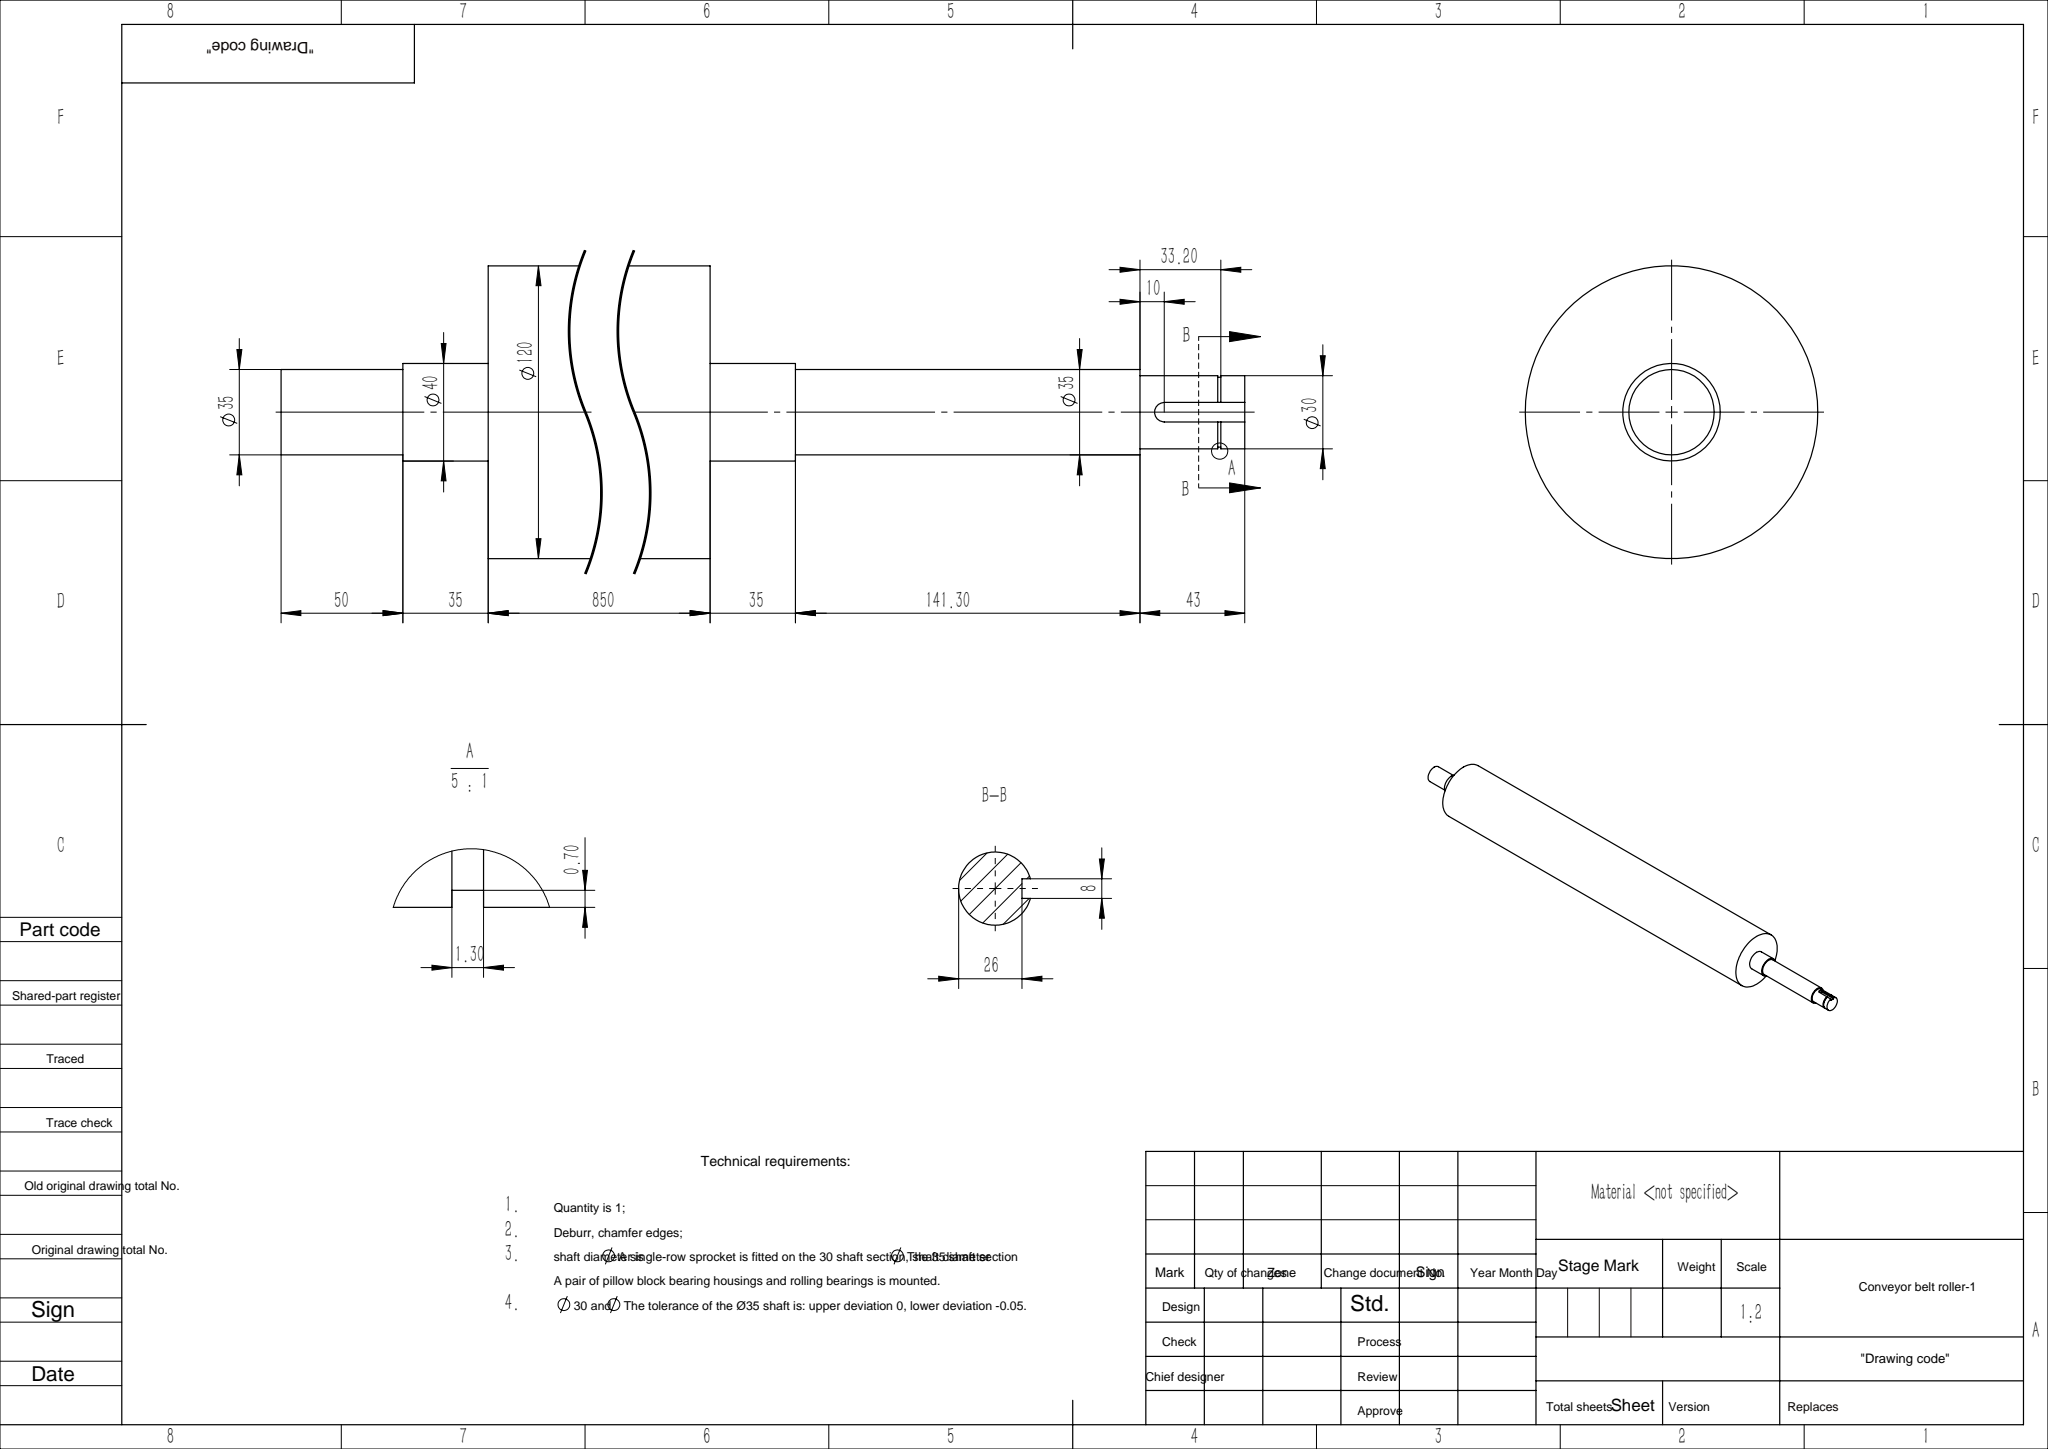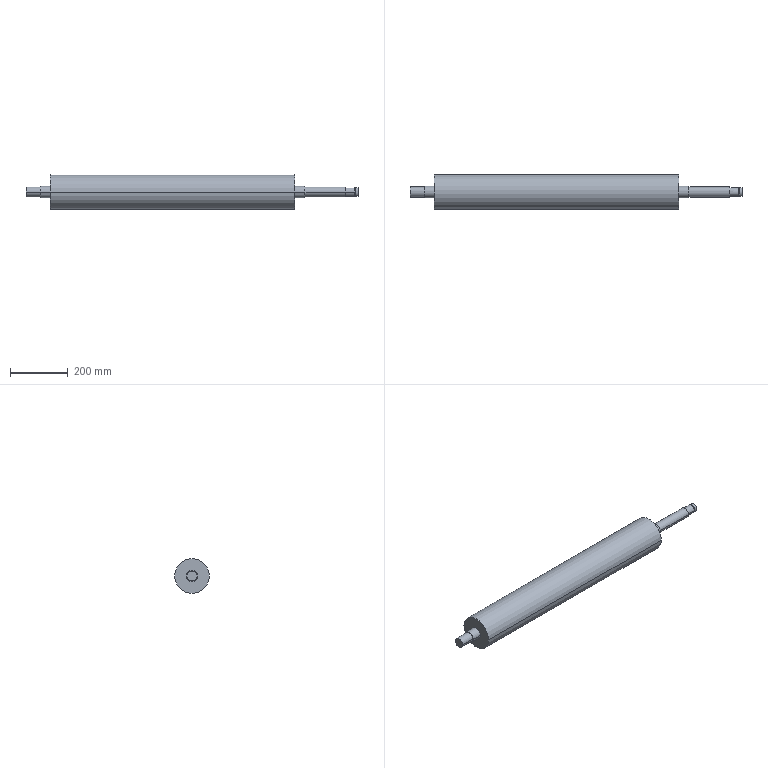Part | SolidWorks | features ICE 2, Revolution 1 | 1 solid | 28 faces | box 1154 x 120 x 120 mm | volume 9914503 mm3 | cylinder 16 | plane 12 | commonest cylinder face diameters 35 x4 40 x4 30 x3 8 x2 120 x2 28.6 x1
STEP:
#1=CARTESIAN_POINT('',(1117.3,11.,0.));
#2=VERTEX_POINT('',#1);
#3=CARTESIAN_POINT('',(1121.3,11.,4.));
#4=VERTEX_POINT('',#3);
#5=CARTESIAN_POINT('',(1121.3,11.,0.));
#6=DIRECTION('',(0.,1.,0.));
#7=DIRECTION('',(-1.,0.,0.));
#8=AXIS2_PLACEMENT_3D('',#5,#6,#7);
#9=CIRCLE('',#8,4.);
#10=EDGE_CURVE('',#2,#4,#9,.T.);
#11=ORIENTED_EDGE('',*,*,#10,.F.);
#12=CARTESIAN_POINT('',(1117.3,15.,0.));
#13=VERTEX_POINT('',#12);
#14=CARTESIAN_POINT('',(1117.3,11.,0.));
#15=DIRECTION('',(0.,1.,0.));
#16=VECTOR('',#15,1000.);
#17=LINE('',#14,#16);
#18=EDGE_CURVE('',#2,#13,#17,.T.);
#19=ORIENTED_EDGE('',*,*,#18,.T.);
#20=CARTESIAN_POINT('',(1121.3,14.457,4.));
#21=VERTEX_POINT('',#20);
#22=CARTESIAN_POINT('',(1117.3,15.,0.));
#23=CARTESIAN_POINT('',(1117.3,15.,0.262));
#24=CARTESIAN_POINT('',(1117.326,14.993,0.5282));
#25=CARTESIAN_POINT('',(1117.429,14.966,1.042));
#26=CARTESIAN_POINT('',(1117.505,14.946,1.292));
#27=CARTESIAN_POINT('',(1117.808,14.871,2.02));
#28=CARTESIAN_POINT('',(1118.102,14.802,2.459));
#29=CARTESIAN_POINT('',(1118.657,14.695,3.014));
#30=CARTESIAN_POINT('',(1118.857,14.66,3.178));
#31=CARTESIAN_POINT('',(1119.289,14.594,3.467));
#32=CARTESIAN_POINT('',(1119.523,14.564,3.593));
#33=CARTESIAN_POINT('',(1120.005,14.513,3.794));
#34=CARTESIAN_POINT('',(1120.254,14.492,3.87));
#35=CARTESIAN_POINT('',(1120.769,14.464,3.973));
#36=CARTESIAN_POINT('',(1121.035,14.457,4.));
#37=CARTESIAN_POINT('',(1121.3,14.457,4.));
#38=B_SPLINE_CURVE_WITH_KNOTS('',3,(#22,#23,#24,#25,#26,#27,#28,#29,#30,#31,#32,#33,#34,#35,#36,#37),.UNSPECIFIED.,.F.,.F.,(4,2,2,2,2,2,2,4),(0.006283,0.007068,0.007852,0.009421,0.01021,0.01099,0.01177,0.01256),.UNSPECIFIED.);
#39=EDGE_CURVE('',#13,#21,#38,.T.);
#40=ORIENTED_EDGE('',*,*,#39,.T.);
#41=CARTESIAN_POINT('',(1121.3,11.,4.));
#42=DIRECTION('',(0.,1.,0.));
#43=VECTOR('',#42,1000.);
#44=LINE('',#41,#43);
#45=EDGE_CURVE('',#4,#21,#44,.T.);
#46=ORIENTED_EDGE('',*,*,#45,.F.);
#47=EDGE_LOOP('',(#11,#19,#40,#46));
#48=FACE_OUTER_BOUND('',#47,.T.);
#49=CARTESIAN_POINT('',(1121.3,11.,0.));
#50=DIRECTION('',(0.,1.,0.));
#51=DIRECTION('',(-1.,0.,0.));
#52=AXIS2_PLACEMENT_3D('',#49,#50,#51);
#53=CYLINDRICAL_SURFACE('',#52,4.);
#54=ADVANCED_FACE('',(#48),#53,.F.);
#55=CARTESIAN_POINT('',(970.,17.5,0.));
#56=VERTEX_POINT('',#55);
#57=CARTESIAN_POINT('',(970.,-17.5,0.));
#58=VERTEX_POINT('',#57);
#59=CARTESIAN_POINT('',(970.,0.,0.));
#60=DIRECTION('',(1.,0.,0.));
#61=DIRECTION('',(0.,1.,0.));
#62=AXIS2_PLACEMENT_3D('',#59,#60,#61);
#63=CIRCLE('',#62,17.5);
#64=EDGE_CURVE('',#56,#58,#63,.T.);
#65=ORIENTED_EDGE('',*,*,#64,.T.);
#66=CARTESIAN_POINT('',(1111.3,-17.5,0.));
#67=VERTEX_POINT('',#66);
#68=CARTESIAN_POINT('',(1154.3,-17.5,0.));
#69=DIRECTION('',(1.,0.,0.));
#70=VECTOR('',#69,1000.);
#71=LINE('',#68,#70);
#72=EDGE_CURVE('',#58,#67,#71,.T.);
#73=ORIENTED_EDGE('',*,*,#72,.T.);
#74=CARTESIAN_POINT('',(1111.3,17.5,0.));
#75=VERTEX_POINT('',#74);
#76=CARTESIAN_POINT('',(1111.3,0.,0.));
#77=DIRECTION('',(1.,0.,0.));
#78=DIRECTION('',(0.,1.,0.));
#79=AXIS2_PLACEMENT_3D('',#76,#77,#78);
#80=CIRCLE('',#79,17.5);
#81=EDGE_CURVE('',#75,#67,#80,.T.);
#82=ORIENTED_EDGE('',*,*,#81,.F.);
#83=CARTESIAN_POINT('',(1154.3,17.5,0.));
#84=DIRECTION('',(1.,0.,0.));
#85=VECTOR('',#84,1000.);
#86=LINE('',#83,#85);
#87=EDGE_CURVE('',#56,#75,#86,.T.);
#88=ORIENTED_EDGE('',*,*,#87,.F.);
#89=EDGE_LOOP('',(#65,#73,#82,#88));
#90=FACE_OUTER_BOUND('',#89,.T.);
#91=CARTESIAN_POINT('',(1154.3,0.,0.));
#92=DIRECTION('',(1.,0.,0.));
#93=DIRECTION('',(0.,1.,0.));
#94=AXIS2_PLACEMENT_3D('',#91,#92,#93);
#95=CYLINDRICAL_SURFACE('',#94,17.5);
#96=ADVANCED_FACE('',(#90),#95,.T.);
#97=CARTESIAN_POINT('',(935.,20.,0.));
#98=VERTEX_POINT('',#97);
#99=CARTESIAN_POINT('',(935.,-20.,0.));
#100=VERTEX_POINT('',#99);
#101=CARTESIAN_POINT('',(935.,0.,0.));
#102=DIRECTION('',(1.,0.,0.));
#103=DIRECTION('',(0.,1.,0.));
#104=AXIS2_PLACEMENT_3D('',#101,#102,#103);
#105=CIRCLE('',#104,20.);
#106=EDGE_CURVE('',#98,#100,#105,.T.);
#107=ORIENTED_EDGE('',*,*,#106,.T.);
#108=CARTESIAN_POINT('',(970.,-20.,0.));
#109=VERTEX_POINT('',#108);
#110=CARTESIAN_POINT('',(1154.3,-20.,0.));
#111=DIRECTION('',(1.,0.,0.));
#112=VECTOR('',#111,1000.);
#113=LINE('',#110,#112);
#114=EDGE_CURVE('',#100,#109,#113,.T.);
#115=ORIENTED_EDGE('',*,*,#114,.T.);
#116=CARTESIAN_POINT('',(970.,20.,0.));
#117=VERTEX_POINT('',#116);
#118=CARTESIAN_POINT('',(970.,0.,0.));
#119=DIRECTION('',(1.,0.,0.));
#120=DIRECTION('',(0.,1.,0.));
#121=AXIS2_PLACEMENT_3D('',#118,#119,#120);
#122=CIRCLE('',#121,20.);
#123=EDGE_CURVE('',#117,#109,#122,.T.);
#124=ORIENTED_EDGE('',*,*,#123,.F.);
#125=CARTESIAN_POINT('',(1154.3,20.,0.));
#126=DIRECTION('',(1.,0.,0.));
#127=VECTOR('',#126,1000.);
#128=LINE('',#125,#127);
#129=EDGE_CURVE('',#98,#117,#128,.T.);
#130=ORIENTED_EDGE('',*,*,#129,.F.);
#131=EDGE_LOOP('',(#107,#115,#124,#130));
#132=FACE_OUTER_BOUND('',#131,.T.);
#133=CARTESIAN_POINT('',(1154.3,0.,0.));
#134=DIRECTION('',(1.,0.,0.));
#135=DIRECTION('',(0.,1.,0.));
#136=AXIS2_PLACEMENT_3D('',#133,#134,#135);
#137=CYLINDRICAL_SURFACE('',#136,20.);
#138=ADVANCED_FACE('',(#132),#137,.T.);
#139=CARTESIAN_POINT('',(85.,60.,0.));
#140=VERTEX_POINT('',#139);
#141=CARTESIAN_POINT('',(85.,-60.,0.));
#142=VERTEX_POINT('',#141);
#143=CARTESIAN_POINT('',(85.,0.,0.));
#144=DIRECTION('',(1.,0.,0.));
#145=DIRECTION('',(0.,1.,0.));
#146=AXIS2_PLACEMENT_3D('',#143,#144,#145);
#147=CIRCLE('',#146,60.);
#148=EDGE_CURVE('',#140,#142,#147,.T.);
#149=ORIENTED_EDGE('',*,*,#148,.T.);
#150=CARTESIAN_POINT('',(935.,-60.,0.));
#151=VERTEX_POINT('',#150);
#152=CARTESIAN_POINT('',(1154.3,-60.,0.));
#153=DIRECTION('',(1.,0.,0.));
#154=VECTOR('',#153,1000.);
#155=LINE('',#152,#154);
#156=EDGE_CURVE('',#142,#151,#155,.T.);
#157=ORIENTED_EDGE('',*,*,#156,.T.);
#158=CARTESIAN_POINT('',(935.,60.,0.));
#159=VERTEX_POINT('',#158);
#160=CARTESIAN_POINT('',(935.,0.,0.));
#161=DIRECTION('',(1.,0.,0.));
#162=DIRECTION('',(0.,1.,0.));
#163=AXIS2_PLACEMENT_3D('',#160,#161,#162);
#164=CIRCLE('',#163,60.);
#165=EDGE_CURVE('',#159,#151,#164,.T.);
#166=ORIENTED_EDGE('',*,*,#165,.F.);
#167=CARTESIAN_POINT('',(1154.3,60.,0.));
#168=DIRECTION('',(1.,0.,0.));
#169=VECTOR('',#168,1000.);
#170=LINE('',#167,#169);
#171=EDGE_CURVE('',#140,#159,#170,.T.);
#172=ORIENTED_EDGE('',*,*,#171,.F.);
#173=EDGE_LOOP('',(#149,#157,#166,#172));
#174=FACE_OUTER_BOUND('',#173,.T.);
#175=CARTESIAN_POINT('',(1154.3,0.,0.));
#176=DIRECTION('',(1.,0.,0.));
#177=DIRECTION('',(0.,1.,0.));
#178=AXIS2_PLACEMENT_3D('',#175,#176,#177);
#179=CYLINDRICAL_SURFACE('',#178,60.);
#180=ADVANCED_FACE('',(#174),#179,.T.);
#181=CARTESIAN_POINT('',(50.,20.,0.));
#182=VERTEX_POINT('',#181);
#183=CARTESIAN_POINT('',(50.,-20.,0.));
#184=VERTEX_POINT('',#183);
#185=CARTESIAN_POINT('',(50.,0.,0.));
#186=DIRECTION('',(1.,0.,0.));
#187=DIRECTION('',(0.,1.,0.));
#188=AXIS2_PLACEMENT_3D('',#185,#186,#187);
#189=CIRCLE('',#188,20.);
#190=EDGE_CURVE('',#182,#184,#189,.T.);
#191=ORIENTED_EDGE('',*,*,#190,.T.);
#192=CARTESIAN_POINT('',(85.,-20.,0.));
#193=VERTEX_POINT('',#192);
#194=CARTESIAN_POINT('',(1154.3,-20.,0.));
#195=DIRECTION('',(1.,0.,0.));
#196=VECTOR('',#195,1000.);
#197=LINE('',#194,#196);
#198=EDGE_CURVE('',#184,#193,#197,.T.);
#199=ORIENTED_EDGE('',*,*,#198,.T.);
#200=CARTESIAN_POINT('',(85.,20.,0.));
#201=VERTEX_POINT('',#200);
#202=CARTESIAN_POINT('',(85.,0.,0.));
#203=DIRECTION('',(1.,0.,0.));
#204=DIRECTION('',(0.,1.,0.));
#205=AXIS2_PLACEMENT_3D('',#202,#203,#204);
#206=CIRCLE('',#205,20.);
#207=EDGE_CURVE('',#201,#193,#206,.T.);
#208=ORIENTED_EDGE('',*,*,#207,.F.);
#209=CARTESIAN_POINT('',(1154.3,20.,0.));
#210=DIRECTION('',(1.,0.,0.));
#211=VECTOR('',#210,1000.);
#212=LINE('',#209,#211);
#213=EDGE_CURVE('',#182,#201,#212,.T.);
#214=ORIENTED_EDGE('',*,*,#213,.F.);
#215=EDGE_LOOP('',(#191,#199,#208,#214));
#216=FACE_OUTER_BOUND('',#215,.T.);
#217=CARTESIAN_POINT('',(1154.3,0.,0.));
#218=DIRECTION('',(1.,0.,0.));
#219=DIRECTION('',(0.,1.,0.));
#220=AXIS2_PLACEMENT_3D('',#217,#218,#219);
#221=CYLINDRICAL_SURFACE('',#220,20.);
#222=ADVANCED_FACE('',(#216),#221,.T.);
#223=CARTESIAN_POINT('',(0.,17.5,0.));
#224=VERTEX_POINT('',#223);
#225=CARTESIAN_POINT('',(0.,-17.5,0.));
#226=VERTEX_POINT('',#225);
#227=CARTESIAN_POINT('',(0.,0.,0.));
#228=DIRECTION('',(1.,0.,0.));
#229=DIRECTION('',(0.,1.,0.));
#230=AXIS2_PLACEMENT_3D('',#227,#228,#229);
#231=CIRCLE('',#230,17.5);
#232=EDGE_CURVE('',#224,#226,#231,.T.);
#233=ORIENTED_EDGE('',*,*,#232,.T.);
#234=CARTESIAN_POINT('',(50.,-17.5,0.));
#235=VERTEX_POINT('',#234);
#236=CARTESIAN_POINT('',(1154.3,-17.5,0.));
#237=DIRECTION('',(1.,0.,0.));
#238=VECTOR('',#237,1000.);
#239=LINE('',#236,#238);
#240=EDGE_CURVE('',#226,#235,#239,.T.);
#241=ORIENTED_EDGE('',*,*,#240,.T.);
#242=CARTESIAN_POINT('',(50.,17.5,0.));
#243=VERTEX_POINT('',#242);
#244=CARTESIAN_POINT('',(50.,0.,0.));
#245=DIRECTION('',(1.,0.,0.));
#246=DIRECTION('',(0.,1.,0.));
#247=AXIS2_PLACEMENT_3D('',#244,#245,#246);
#248=CIRCLE('',#247,17.5);
#249=EDGE_CURVE('',#243,#235,#248,.T.);
#250=ORIENTED_EDGE('',*,*,#249,.F.);
#251=CARTESIAN_POINT('',(1154.3,17.5,0.));
#252=DIRECTION('',(1.,0.,0.));
#253=VECTOR('',#252,1000.);
#254=LINE('',#251,#253);
#255=EDGE_CURVE('',#224,#243,#254,.T.);
#256=ORIENTED_EDGE('',*,*,#255,.F.);
#257=EDGE_LOOP('',(#233,#241,#250,#256));
#258=FACE_OUTER_BOUND('',#257,.T.);
#259=CARTESIAN_POINT('',(1154.3,0.,0.));
#260=DIRECTION('',(1.,0.,0.));
#261=DIRECTION('',(0.,1.,0.));
#262=AXIS2_PLACEMENT_3D('',#259,#260,#261);
#263=CYLINDRICAL_SURFACE('',#262,17.5);
#264=ADVANCED_FACE('',(#258),#263,.T.);
#265=CARTESIAN_POINT('',(1111.3,15.,0.));
#266=VERTEX_POINT('',#265);
#267=CARTESIAN_POINT('',(1111.3,-15.,0.));
#268=VERTEX_POINT('',#267);
#269=CARTESIAN_POINT('',(1111.3,0.,0.));
#270=DIRECTION('',(1.,0.,0.));
#271=DIRECTION('',(0.,1.,0.));
#272=AXIS2_PLACEMENT_3D('',#269,#270,#271);
#273=CIRCLE('',#272,15.);
#274=EDGE_CURVE('',#266,#268,#273,.T.);
#275=ORIENTED_EDGE('',*,*,#274,.T.);
#276=CARTESIAN_POINT('',(1143.2,-15.,0.));
#277=VERTEX_POINT('',#276);
#278=CARTESIAN_POINT('',(1154.3,-15.,0.));
#279=DIRECTION('',(1.,0.,0.));
#280=VECTOR('',#279,1000.);
#281=LINE('',#278,#280);
#282=EDGE_CURVE('',#268,#277,#281,.T.);
#283=ORIENTED_EDGE('',*,*,#282,.T.);
#284=CARTESIAN_POINT('',(1143.2,14.457,4.));
#285=VERTEX_POINT('',#284);
#286=CARTESIAN_POINT('',(1143.2,0.,0.));
#287=DIRECTION('',(1.,0.,0.));
#288=DIRECTION('',(0.,1.,0.));
#289=AXIS2_PLACEMENT_3D('',#286,#287,#288);
#290=CIRCLE('',#289,15.);
#291=EDGE_CURVE('',#285,#277,#290,.T.);
#292=ORIENTED_EDGE('',*,*,#291,.F.);
#293=CARTESIAN_POINT('',(1154.3,14.457,4.));
#294=DIRECTION('',(1.,0.,0.));
#295=VECTOR('',#294,1000.);
#296=LINE('',#293,#295);
#297=EDGE_CURVE('',#21,#285,#296,.T.);
#298=ORIENTED_EDGE('',*,*,#297,.F.);
#299=ORIENTED_EDGE('',*,*,#39,.F.);
#300=CARTESIAN_POINT('',(1154.3,15.,0.));
#301=DIRECTION('',(1.,0.,0.));
#302=VECTOR('',#301,1000.);
#303=LINE('',#300,#302);
#304=EDGE_CURVE('',#266,#13,#303,.T.);
#305=ORIENTED_EDGE('',*,*,#304,.F.);
#306=EDGE_LOOP('',(#275,#283,#292,#298,#299,#305));
#307=FACE_OUTER_BOUND('',#306,.T.);
#308=CARTESIAN_POINT('',(1154.3,0.,0.));
#309=DIRECTION('',(1.,0.,0.));
#310=DIRECTION('',(0.,1.,0.));
#311=AXIS2_PLACEMENT_3D('',#308,#309,#310);
#312=CYLINDRICAL_SURFACE('',#311,15.);
#313=ADVANCED_FACE('',(#307),#312,.T.);
#314=ORIENTED_EDGE('',*,*,#282,.F.);
#315=CARTESIAN_POINT('',(1111.3,0.,0.));
#316=DIRECTION('',(1.,0.,0.));
#317=DIRECTION('',(0.,1.,0.));
#318=AXIS2_PLACEMENT_3D('',#315,#316,#317);
#319=CIRCLE('',#318,15.);
#320=EDGE_CURVE('',#268,#266,#319,.T.);
#321=ORIENTED_EDGE('',*,*,#320,.T.);
#322=ORIENTED_EDGE('',*,*,#304,.T.);
#323=CARTESIAN_POINT('',(1121.3,14.457,-4.));
#324=VERTEX_POINT('',#323);
#325=CARTESIAN_POINT('',(1121.3,14.457,-4.));
#326=CARTESIAN_POINT('',(1121.034,14.457,-4.));
#327=CARTESIAN_POINT('',(1120.773,14.464,-3.974));
#328=CARTESIAN_POINT('',(1120.26,14.492,-3.871));
#329=CARTESIAN_POINT('',(1120.006,14.513,-3.794));
#330=CARTESIAN_POINT('',(1119.522,14.564,-3.593));
#331=CARTESIAN_POINT('',(1119.292,14.594,-3.47));
#332=CARTESIAN_POINT('',(1118.858,14.66,-3.179));
#333=CARTESIAN_POINT('',(1118.654,14.696,-3.011));
#334=CARTESIAN_POINT('',(1118.287,14.766,-2.644));
#335=CARTESIAN_POINT('',(1118.122,14.801,-2.443));
#336=CARTESIAN_POINT('',(1117.829,14.867,-2.006));
#337=CARTESIAN_POINT('',(1117.706,14.897,-1.775));
#338=CARTESIAN_POINT('',(1117.506,14.946,-1.293));
#339=CARTESIAN_POINT('',(1117.429,14.966,-1.04));
#340=CARTESIAN_POINT('',(1117.326,14.993,-0.5228));
#341=CARTESIAN_POINT('',(1117.3,15.,-0.2623));
#342=CARTESIAN_POINT('',(1117.3,15.,0.));
#343=B_SPLINE_CURVE_WITH_KNOTS('',3,(#325,#326,#327,#328,#329,#330,#331,#332,#333,#334,#335,#336,#337,#338,#339,#340,#341,#342),.UNSPECIFIED.,.F.,.F.,(4,2,2,2,2,2,2,2,4),(0.,0.0007854,0.001571,0.002356,0.003142,0.003927,0.004712,0.005498,0.006283),.UNSPECIFIED.);
#344=EDGE_CURVE('',#324,#13,#343,.T.);
#345=ORIENTED_EDGE('',*,*,#344,.F.);
#346=CARTESIAN_POINT('',(1143.2,14.457,-4.));
#347=VERTEX_POINT('',#346);
#348=CARTESIAN_POINT('',(1154.3,14.457,-4.));
#349=DIRECTION('',(-1.,0.,0.));
#350=VECTOR('',#349,1000.);
#351=LINE('',#348,#350);
#352=EDGE_CURVE('',#347,#324,#351,.T.);
#353=ORIENTED_EDGE('',*,*,#352,.F.);
#354=CARTESIAN_POINT('',(1143.2,0.,0.));
#355=DIRECTION('',(1.,0.,0.));
#356=DIRECTION('',(0.,1.,0.));
#357=AXIS2_PLACEMENT_3D('',#354,#355,#356);
#358=CIRCLE('',#357,15.);
#359=EDGE_CURVE('',#277,#347,#358,.T.);
#360=ORIENTED_EDGE('',*,*,#359,.F.);
#361=EDGE_LOOP('',(#314,#321,#322,#345,#353,#360));
#362=FACE_OUTER_BOUND('',#361,.T.);
#363=CARTESIAN_POINT('',(1154.3,0.,0.));
#364=DIRECTION('',(1.,0.,0.));
#365=DIRECTION('',(0.,1.,0.));
#366=AXIS2_PLACEMENT_3D('',#363,#364,#365);
#367=CYLINDRICAL_SURFACE('',#366,15.);
#368=ADVANCED_FACE('',(#362),#367,.T.);
#369=CARTESIAN_POINT('',(1143.2,13.729,-4.));
#370=VERTEX_POINT('',#369);
#371=CARTESIAN_POINT('',(1143.2,11.,-4.));
#372=DIRECTION('',(0.,-1.,0.));
#373=VECTOR('',#372,1000.);
#374=LINE('',#371,#373);
#375=EDGE_CURVE('',#347,#370,#374,.T.);
#376=ORIENTED_EDGE('',*,*,#375,.F.);
#377=ORIENTED_EDGE('',*,*,#352,.T.);
#378=CARTESIAN_POINT('',(1121.3,11.,-4.));
#379=VERTEX_POINT('',#378);
#380=CARTESIAN_POINT('',(1121.3,11.,-4.));
#381=DIRECTION('',(0.,1.,0.));
#382=VECTOR('',#381,1000.);
#383=LINE('',#380,#382);
#384=EDGE_CURVE('',#379,#324,#383,.T.);
#385=ORIENTED_EDGE('',*,*,#384,.F.);
#386=CARTESIAN_POINT('',(1154.3,11.,-4.));
#387=VERTEX_POINT('',#386);
#388=CARTESIAN_POINT('',(1121.3,11.,-4.));
#389=DIRECTION('',(-1.,0.,0.));
#390=VECTOR('',#389,1000.);
#391=LINE('',#388,#390);
#392=EDGE_CURVE('',#387,#379,#391,.T.);
#393=ORIENTED_EDGE('',*,*,#392,.F.);
#394=CARTESIAN_POINT('',(1154.3,14.457,-4.));
#395=VERTEX_POINT('',#394);
#396=CARTESIAN_POINT('',(1154.3,15.,-4.));
#397=DIRECTION('',(0.,1.,0.));
#398=VECTOR('',#397,1000.);
#399=LINE('',#396,#398);
#400=EDGE_CURVE('',#387,#395,#399,.T.);
#401=ORIENTED_EDGE('',*,*,#400,.T.);
#402=CARTESIAN_POINT('',(1144.5,14.457,-4.));
#403=VERTEX_POINT('',#402);
#404=CARTESIAN_POINT('',(1154.3,14.457,-4.));
#405=DIRECTION('',(-1.,0.,0.));
#406=VECTOR('',#405,1000.);
#407=LINE('',#404,#406);
#408=EDGE_CURVE('',#395,#403,#407,.T.);
#409=ORIENTED_EDGE('',*,*,#408,.T.);
#410=CARTESIAN_POINT('',(1144.5,13.729,-4.));
#411=VERTEX_POINT('',#410);
#412=CARTESIAN_POINT('',(1144.5,11.,-4.));
#413=DIRECTION('',(0.,-1.,0.));
#414=VECTOR('',#413,1000.);
#415=LINE('',#412,#414);
#416=EDGE_CURVE('',#403,#411,#415,.T.);
#417=ORIENTED_EDGE('',*,*,#416,.T.);
#418=CARTESIAN_POINT('',(1143.2,13.729,-4.));
#419=DIRECTION('',(1.,0.,0.));
#420=VECTOR('',#419,1000.);
#421=LINE('',#418,#420);
#422=EDGE_CURVE('',#370,#411,#421,.T.);
#423=ORIENTED_EDGE('',*,*,#422,.F.);
#424=EDGE_LOOP('',(#376,#377,#385,#393,#401,#409,#417,#423));
#425=FACE_OUTER_BOUND('',#424,.T.);
#426=CARTESIAN_POINT('',(1121.3,11.,-4.));
#427=DIRECTION('',(0.,0.,-1.));
#428=DIRECTION('',(-1.,0.,0.));
#429=AXIS2_PLACEMENT_3D('',#426,#427,#428);
#430=PLANE('',#429);
#431=ADVANCED_FACE('',(#425),#430,.F.);
#432=CARTESIAN_POINT('',(1143.2,13.729,4.));
#433=VERTEX_POINT('',#432);
#434=CARTESIAN_POINT('',(1143.2,11.,4.));
#435=DIRECTION('',(0.,1.,0.));
#436=VECTOR('',#435,1000.);
#437=LINE('',#434,#436);
#438=EDGE_CURVE('',#433,#285,#437,.T.);
#439=ORIENTED_EDGE('',*,*,#438,.F.);
#440=CARTESIAN_POINT('',(1144.5,13.729,4.));
#441=VERTEX_POINT('',#440);
#442=CARTESIAN_POINT('',(1143.2,13.729,4.));
#443=DIRECTION('',(-1.,0.,0.));
#444=VECTOR('',#443,1000.);
#445=LINE('',#442,#444);
#446=EDGE_CURVE('',#441,#433,#445,.T.);
#447=ORIENTED_EDGE('',*,*,#446,.F.);
#448=CARTESIAN_POINT('',(1144.5,14.457,4.));
#449=VERTEX_POINT('',#448);
#450=CARTESIAN_POINT('',(1144.5,11.,4.));
#451=DIRECTION('',(0.,1.,0.));
#452=VECTOR('',#451,1000.);
#453=LINE('',#450,#452);
#454=EDGE_CURVE('',#441,#449,#453,.T.);
#455=ORIENTED_EDGE('',*,*,#454,.T.);
#456=CARTESIAN_POINT('',(1154.3,14.457,4.));
#457=VERTEX_POINT('',#456);
#458=CARTESIAN_POINT('',(1154.3,14.457,4.));
#459=DIRECTION('',(1.,0.,0.));
#460=VECTOR('',#459,1000.);
#461=LINE('',#458,#460);
#462=EDGE_CURVE('',#449,#457,#461,.T.);
#463=ORIENTED_EDGE('',*,*,#462,.T.);
#464=CARTESIAN_POINT('',(1154.3,11.,4.));
#465=VERTEX_POINT('',#464);
#466=CARTESIAN_POINT('',(1154.3,15.,4.));
#467=DIRECTION('',(0.,-1.,0.));
#468=VECTOR('',#467,1000.);
#469=LINE('',#466,#468);
#470=EDGE_CURVE('',#457,#465,#469,.T.);
#471=ORIENTED_EDGE('',*,*,#470,.T.);
#472=CARTESIAN_POINT('',(1121.3,11.,4.));
#473=DIRECTION('',(1.,0.,0.));
#474=VECTOR('',#473,1000.);
#475=LINE('',#472,#474);
#476=EDGE_CURVE('',#4,#465,#475,.T.);
#477=ORIENTED_EDGE('',*,*,#476,.F.);
#478=ORIENTED_EDGE('',*,*,#45,.T.);
#479=ORIENTED_EDGE('',*,*,#297,.T.);
#480=EDGE_LOOP('',(#439,#447,#455,#463,#471,#477,#478,#479));
#481=FACE_OUTER_BOUND('',#480,.T.);
#482=CARTESIAN_POINT('',(1121.3,11.,4.));
#483=DIRECTION('',(0.,0.,1.));
#484=DIRECTION('',(1.,0.,0.));
#485=AXIS2_PLACEMENT_3D('',#482,#483,#484);
#486=PLANE('',#485);
#487=ADVANCED_FACE('',(#481),#486,.F.);
#488=ORIENTED_EDGE('',*,*,#232,.F.);
#489=CARTESIAN_POINT('',(0.,0.,0.));
#490=DIRECTION('',(1.,0.,0.));
#491=DIRECTION('',(0.,1.,0.));
#492=AXIS2_PLACEMENT_3D('',#489,#490,#491);
#493=CIRCLE('',#492,17.5);
#494=EDGE_CURVE('',#226,#224,#493,.T.);
#495=ORIENTED_EDGE('',*,*,#494,.F.);
#496=EDGE_LOOP('',(#488,#495));
#497=FACE_OUTER_BOUND('',#496,.T.);
#498=CARTESIAN_POINT('',(0.,0.,0.));
#499=DIRECTION('',(-1.,0.,0.));
#500=DIRECTION('',(0.,-1.,0.));
#501=AXIS2_PLACEMENT_3D('',#498,#499,#500);
#502=PLANE('',#501);
#503=ADVANCED_FACE('',(#497),#502,.T.);
#504=ORIENTED_EDGE('',*,*,#240,.F.);
#505=ORIENTED_EDGE('',*,*,#494,.T.);
#506=ORIENTED_EDGE('',*,*,#255,.T.);
#507=CARTESIAN_POINT('',(50.,0.,0.));
#508=DIRECTION('',(1.,0.,0.));
#509=DIRECTION('',(0.,1.,0.));
#510=AXIS2_PLACEMENT_3D('',#507,#508,#509);
#511=CIRCLE('',#510,17.5);
#512=EDGE_CURVE('',#235,#243,#511,.T.);
#513=ORIENTED_EDGE('',*,*,#512,.F.);
#514=EDGE_LOOP('',(#504,#505,#506,#513));
#515=FACE_OUTER_BOUND('',#514,.T.);
#516=CARTESIAN_POINT('',(1154.3,0.,0.));
#517=DIRECTION('',(1.,0.,0.));
#518=DIRECTION('',(0.,1.,0.));
#519=AXIS2_PLACEMENT_3D('',#516,#517,#518);
#520=CYLINDRICAL_SURFACE('',#519,17.5);
#521=ADVANCED_FACE('',(#515),#520,.T.);
#522=ORIENTED_EDGE('',*,*,#249,.T.);
#523=ORIENTED_EDGE('',*,*,#512,.T.);
#524=EDGE_LOOP('',(#522,#523));
#525=FACE_BOUND('',#524,.T.);
#526=ORIENTED_EDGE('',*,*,#190,.F.);
#527=CARTESIAN_POINT('',(50.,0.,0.));
#528=DIRECTION('',(1.,0.,0.));
#529=DIRECTION('',(0.,1.,0.));
#530=AXIS2_PLACEMENT_3D('',#527,#528,#529);
#531=CIRCLE('',#530,20.);
#532=EDGE_CURVE('',#184,#182,#531,.T.);
#533=ORIENTED_EDGE('',*,*,#532,.F.);
#534=EDGE_LOOP('',(#526,#533));
#535=FACE_OUTER_BOUND('',#534,.T.);
#536=CARTESIAN_POINT('',(50.,17.5,0.));
#537=DIRECTION('',(-1.,0.,0.));
#538=DIRECTION('',(0.,-1.,0.));
#539=AXIS2_PLACEMENT_3D('',#536,#537,#538);
#540=PLANE('',#539);
#541=ADVANCED_FACE('',(#525,#535),#540,.T.);
#542=ORIENTED_EDGE('',*,*,#198,.F.);
#543=ORIENTED_EDGE('',*,*,#532,.T.);
#544=ORIENTED_EDGE('',*,*,#213,.T.);
#545=CARTESIAN_POINT('',(85.,0.,0.));
#546=DIRECTION('',(1.,0.,0.));
#547=DIRECTION('',(0.,1.,0.));
#548=AXIS2_PLACEMENT_3D('',#545,#546,#547);
#549=CIRCLE('',#548,20.);
#550=EDGE_CURVE('',#193,#201,#549,.T.);
#551=ORIENTED_EDGE('',*,*,#550,.F.);
#552=EDGE_LOOP('',(#542,#543,#544,#551));
#553=FACE_OUTER_BOUND('',#552,.T.);
#554=CARTESIAN_POINT('',(1154.3,0.,0.));
#555=DIRECTION('',(1.,0.,0.));
#556=DIRECTION('',(0.,1.,0.));
#557=AXIS2_PLACEMENT_3D('',#554,#555,#556);
#558=CYLINDRICAL_SURFACE('',#557,20.);
#559=ADVANCED_FACE('',(#553),#558,.T.);
#560=ORIENTED_EDGE('',*,*,#207,.T.);
#561=ORIENTED_EDGE('',*,*,#550,.T.);
#562=EDGE_LOOP('',(#560,#561));
#563=FACE_BOUND('',#562,.T.);
#564=ORIENTED_EDGE('',*,*,#148,.F.);
#565=CARTESIAN_POINT('',(85.,0.,0.));
#566=DIRECTION('',(1.,0.,0.));
#567=DIRECTION('',(0.,1.,0.));
#568=AXIS2_PLACEMENT_3D('',#565,#566,#567);
#569=CIRCLE('',#568,60.);
#570=EDGE_CURVE('',#142,#140,#569,.T.);
#571=ORIENTED_EDGE('',*,*,#570,.F.);
#572=EDGE_LOOP('',(#564,#571));
#573=FACE_OUTER_BOUND('',#572,.T.);
#574=CARTESIAN_POINT('',(85.,20.,0.));
#575=DIRECTION('',(-1.,0.,0.));
#576=DIRECTION('',(0.,-1.,0.));
#577=AXIS2_PLACEMENT_3D('',#574,#575,#576);
#578=PLANE('',#577);
#579=ADVANCED_FACE('',(#563,#573),#578,.T.);
#580=ORIENTED_EDGE('',*,*,#156,.F.);
#581=ORIENTED_EDGE('',*,*,#570,.T.);
#582=ORIENTED_EDGE('',*,*,#171,.T.);
#583=CARTESIAN_POINT('',(935.,0.,0.));
#584=DIRECTION('',(1.,0.,0.));
#585=DIRECTION('',(0.,1.,0.));
#586=AXIS2_PLACEMENT_3D('',#583,#584,#585);
#587=CIRCLE('',#586,60.);
#588=EDGE_CURVE('',#151,#159,#587,.T.);
#589=ORIENTED_EDGE('',*,*,#588,.F.);
#590=EDGE_LOOP('',(#580,#581,#582,#589));
#591=FACE_OUTER_BOUND('',#590,.T.);
#592=CARTESIAN_POINT('',(1154.3,0.,0.));
#593=DIRECTION('',(1.,0.,0.));
#594=DIRECTION('',(0.,1.,0.));
#595=AXIS2_PLACEMENT_3D('',#592,#593,#594);
#596=CYLINDRICAL_SURFACE('',#595,60.);
#597=ADVANCED_FACE('',(#591),#596,.T.);
#598=ORIENTED_EDGE('',*,*,#165,.T.);
#599=ORIENTED_EDGE('',*,*,#588,.T.);
#600=EDGE_LOOP('',(#598,#599));
#601=FACE_OUTER_BOUND('',#600,.T.);
#602=ORIENTED_EDGE('',*,*,#106,.F.);
#603=CARTESIAN_POINT('',(935.,0.,0.));
#604=DIRECTION('',(1.,0.,0.));
#605=DIRECTION('',(0.,1.,0.));
#606=AXIS2_PLACEMENT_3D('',#603,#604,#605);
#607=CIRCLE('',#606,20.);
#608=EDGE_CURVE('',#100,#98,#607,.T.);
#609=ORIENTED_EDGE('',*,*,#608,.F.);
#610=EDGE_LOOP('',(#602,#609));
#611=FACE_BOUND('',#610,.T.);
#612=CARTESIAN_POINT('',(935.,60.,0.));
#613=DIRECTION('',(1.,0.,0.));
#614=DIRECTION('',(0.,1.,0.));
#615=AXIS2_PLACEMENT_3D('',#612,#613,#614);
#616=PLANE('',#615);
#617=ADVANCED_FACE('',(#601,#611),#616,.T.);
#618=ORIENTED_EDGE('',*,*,#114,.F.);
#619=ORIENTED_EDGE('',*,*,#608,.T.);
#620=ORIENTED_EDGE('',*,*,#129,.T.);
#621=CARTESIAN_POINT('',(970.,0.,0.));
#622=DIRECTION('',(1.,0.,0.));
#623=DIRECTION('',(0.,1.,0.));
#624=AXIS2_PLACEMENT_3D('',#621,#622,#623);
#625=CIRCLE('',#624,20.);
#626=EDGE_CURVE('',#109,#117,#625,.T.);
#627=ORIENTED_EDGE('',*,*,#626,.F.);
#628=EDGE_LOOP('',(#618,#619,#620,#627));
#629=FACE_OUTER_BOUND('',#628,.T.);
#630=CARTESIAN_POINT('',(1154.3,0.,0.));
#631=DIRECTION('',(1.,0.,0.));
#632=DIRECTION('',(0.,1.,0.));
#633=AXIS2_PLACEMENT_3D('',#630,#631,#632);
#634=CYLINDRICAL_SURFACE('',#633,20.);
#635=ADVANCED_FACE('',(#629),#634,.T.);
#636=ORIENTED_EDGE('',*,*,#123,.T.);
#637=ORIENTED_EDGE('',*,*,#626,.T.);
#638=EDGE_LOOP('',(#636,#637));
#639=FACE_OUTER_BOUND('',#638,.T.);
#640=ORIENTED_EDGE('',*,*,#64,.F.);
#641=CARTESIAN_POINT('',(970.,0.,0.));
#642=DIRECTION('',(1.,0.,0.));
#643=DIRECTION('',(0.,1.,0.));
#644=AXIS2_PLACEMENT_3D('',#641,#642,#643);
#645=CIRCLE('',#644,17.5);
#646=EDGE_CURVE('',#58,#56,#645,.T.);
#647=ORIENTED_EDGE('',*,*,#646,.F.);
#648=EDGE_LOOP('',(#640,#647));
#649=FACE_BOUND('',#648,.T.);
#650=CARTESIAN_POINT('',(970.,20.,0.));
#651=DIRECTION('',(1.,0.,0.));
#652=DIRECTION('',(0.,1.,0.));
#653=AXIS2_PLACEMENT_3D('',#650,#651,#652);
#654=PLANE('',#653);
#655=ADVANCED_FACE('',(#639,#649),#654,.T.);
#656=ORIENTED_EDGE('',*,*,#72,.F.);
#657=ORIENTED_EDGE('',*,*,#646,.T.);
#658=ORIENTED_EDGE('',*,*,#87,.T.);
#659=CARTESIAN_POINT('',(1111.3,0.,0.));
#660=DIRECTION('',(1.,0.,0.));
#661=DIRECTION('',(0.,1.,0.));
#662=AXIS2_PLACEMENT_3D('',#659,#660,#661);
#663=CIRCLE('',#662,17.5);
#664=EDGE_CURVE('',#67,#75,#663,.T.);
#665=ORIENTED_EDGE('',*,*,#664,.F.);
#666=EDGE_LOOP('',(#656,#657,#658,#665));
#667=FACE_OUTER_BOUND('',#666,.T.);
#668=CARTESIAN_POINT('',(1154.3,0.,0.));
#669=DIRECTION('',(1.,0.,0.));
#670=DIRECTION('',(0.,1.,0.));
#671=AXIS2_PLACEMENT_3D('',#668,#669,#670);
#672=CYLINDRICAL_SURFACE('',#671,17.5);
#673=ADVANCED_FACE('',(#667),#672,.T.);
#674=ORIENTED_EDGE('',*,*,#81,.T.);
#675=ORIENTED_EDGE('',*,*,#664,.T.);
#676=EDGE_LOOP('',(#674,#675));
#677=FACE_OUTER_BOUND('',#676,.T.);
#678=ORIENTED_EDGE('',*,*,#274,.F.);
#679=ORIENTED_EDGE('',*,*,#320,.F.);
#680=EDGE_LOOP('',(#678,#679));
#681=FACE_BOUND('',#680,.T.);
#682=CARTESIAN_POINT('',(1111.3,17.5,0.));
#683=DIRECTION('',(1.,0.,0.));
#684=DIRECTION('',(0.,1.,0.));
#685=AXIS2_PLACEMENT_3D('',#682,#683,#684);
#686=PLANE('',#685);
#687=ADVANCED_FACE('',(#677,#681),#686,.T.);
#688=CARTESIAN_POINT('',(1144.5,0.,0.));
#689=DIRECTION('',(1.,0.,0.));
#690=DIRECTION('',(0.,1.,0.));
#691=AXIS2_PLACEMENT_3D('',#688,#689,#690);
#692=CIRCLE('',#691,15.);
#693=EDGE_CURVE('',#449,#403,#692,.T.);
#694=ORIENTED_EDGE('',*,*,#693,.T.);
#695=ORIENTED_EDGE('',*,*,#408,.F.);
#696=CARTESIAN_POINT('',(1154.3,0.,0.));
#697=DIRECTION('',(1.,0.,0.));
#698=DIRECTION('',(0.,1.,0.));
#699=AXIS2_PLACEMENT_3D('',#696,#697,#698);
#700=CIRCLE('',#699,15.);
#701=EDGE_CURVE('',#457,#395,#700,.T.);
#702=ORIENTED_EDGE('',*,*,#701,.F.);
#703=ORIENTED_EDGE('',*,*,#462,.F.);
#704=EDGE_LOOP('',(#694,#695,#702,#703));
#705=FACE_OUTER_BOUND('',#704,.T.);
#706=CARTESIAN_POINT('',(1154.3,0.,0.));
#707=DIRECTION('',(1.,0.,0.));
#708=DIRECTION('',(0.,1.,0.));
#709=AXIS2_PLACEMENT_3D('',#706,#707,#708);
#710=CYLINDRICAL_SURFACE('',#709,15.);
#711=ADVANCED_FACE('',(#705),#710,.T.);
#712=ORIENTED_EDGE('',*,*,#400,.F.);
#713=CARTESIAN_POINT('',(1154.3,11.,0.));
#714=DIRECTION('',(0.,0.,1.));
#715=VECTOR('',#714,1000.);
#716=LINE('',#713,#715);
#717=EDGE_CURVE('',#387,#465,#716,.T.);
#718=ORIENTED_EDGE('',*,*,#717,.T.);
#719=ORIENTED_EDGE('',*,*,#470,.F.);
#720=ORIENTED_EDGE('',*,*,#701,.T.);
#721=EDGE_LOOP('',(#712,#718,#719,#720));
#722=FACE_OUTER_BOUND('',#721,.T.);
#723=CARTESIAN_POINT('',(1154.3,15.,0.));
#724=DIRECTION('',(1.,0.,0.));
#725=DIRECTION('',(0.,1.,0.));
#726=AXIS2_PLACEMENT_3D('',#723,#724,#725);
#727=PLANE('',#726);
#728=ADVANCED_FACE('',(#722),#727,.T.);
#729=ORIENTED_EDGE('',*,*,#18,.F.);
#730=CARTESIAN_POINT('',(1121.3,11.,0.));
#731=DIRECTION('',(0.,1.,0.));
#732=DIRECTION('',(-1.,0.,0.));
#733=AXIS2_PLACEMENT_3D('',#730,#731,#732);
#734=CIRCLE('',#733,4.);
#735=EDGE_CURVE('',#379,#2,#734,.T.);
#736=ORIENTED_EDGE('',*,*,#735,.F.);
#737=ORIENTED_EDGE('',*,*,#384,.T.);
#738=ORIENTED_EDGE('',*,*,#344,.T.);
#739=EDGE_LOOP('',(#729,#736,#737,#738));
#740=FACE_OUTER_BOUND('',#739,.T.);
#741=CARTESIAN_POINT('',(1121.3,11.,0.));
#742=DIRECTION('',(0.,1.,0.));
#743=DIRECTION('',(-1.,0.,0.));
#744=AXIS2_PLACEMENT_3D('',#741,#742,#743);
#745=CYLINDRICAL_SURFACE('',#744,4.);
#746=ADVANCED_FACE('',(#740),#745,.F.);
#747=ORIENTED_EDGE('',*,*,#392,.T.);
#748=ORIENTED_EDGE('',*,*,#735,.T.);
#749=ORIENTED_EDGE('',*,*,#10,.T.);
#750=ORIENTED_EDGE('',*,*,#476,.T.);
#751=ORIENTED_EDGE('',*,*,#717,.F.);
#752=EDGE_LOOP('',(#747,#748,#749,#750,#751));
#753=FACE_OUTER_BOUND('',#752,.T.);
#754=CARTESIAN_POINT('',(1121.3,11.,0.));
#755=DIRECTION('',(0.,1.,0.));
#756=DIRECTION('',(-1.,0.,0.));
#757=AXIS2_PLACEMENT_3D('',#754,#755,#756);
#758=PLANE('',#757);
#759=ADVANCED_FACE('',(#753),#758,.T.);
#760=ORIENTED_EDGE('',*,*,#375,.T.);
#761=CARTESIAN_POINT('',(1143.2,0.,0.));
#762=DIRECTION('',(1.,0.,0.));
#763=DIRECTION('',(0.,1.,0.));
#764=AXIS2_PLACEMENT_3D('',#761,#762,#763);
#765=CIRCLE('',#764,14.3);
#766=EDGE_CURVE('',#433,#370,#765,.T.);
#767=ORIENTED_EDGE('',*,*,#766,.F.);
#768=ORIENTED_EDGE('',*,*,#438,.T.);
#769=ORIENTED_EDGE('',*,*,#291,.T.);
#770=ORIENTED_EDGE('',*,*,#359,.T.);
#771=EDGE_LOOP('',(#760,#767,#768,#769,#770));
#772=FACE_OUTER_BOUND('',#771,.T.);
#773=CARTESIAN_POINT('',(1143.2,0.,0.));
#774=DIRECTION('',(1.,0.,0.));
#775=DIRECTION('',(0.,1.,0.));
#776=AXIS2_PLACEMENT_3D('',#773,#774,#775);
#777=PLANE('',#776);
#778=ADVANCED_FACE('',(#772),#777,.T.);
#779=ORIENTED_EDGE('',*,*,#693,.F.);
#780=ORIENTED_EDGE('',*,*,#454,.F.);
#781=CARTESIAN_POINT('',(1144.5,0.,0.));
#782=DIRECTION('',(1.,0.,0.));
#783=DIRECTION('',(0.,1.,0.));
#784=AXIS2_PLACEMENT_3D('',#781,#782,#783);
#785=CIRCLE('',#784,14.3);
#786=EDGE_CURVE('',#441,#411,#785,.T.);
#787=ORIENTED_EDGE('',*,*,#786,.T.);
#788=ORIENTED_EDGE('',*,*,#416,.F.);
#789=EDGE_LOOP('',(#779,#780,#787,#788));
#790=FACE_OUTER_BOUND('',#789,.T.);
#791=CARTESIAN_POINT('',(1144.5,0.,0.));
#792=DIRECTION('',(1.,0.,0.));
#793=DIRECTION('',(0.,1.,0.));
#794=AXIS2_PLACEMENT_3D('',#791,#792,#793);
#795=PLANE('',#794);
#796=ADVANCED_FACE('',(#790),#795,.F.);
#797=ORIENTED_EDGE('',*,*,#422,.T.);
#798=ORIENTED_EDGE('',*,*,#786,.F.);
#799=ORIENTED_EDGE('',*,*,#446,.T.);
#800=ORIENTED_EDGE('',*,*,#766,.T.);
#801=EDGE_LOOP('',(#797,#798,#799,#800));
#802=FACE_OUTER_BOUND('',#801,.T.);
#803=CARTESIAN_POINT('',(1143.2,0.,0.));
#804=DIRECTION('',(1.,0.,0.));
#805=DIRECTION('',(0.,1.,0.));
#806=AXIS2_PLACEMENT_3D('',#803,#804,#805);
#807=CYLINDRICAL_SURFACE('',#806,14.3);
#808=ADVANCED_FACE('',(#802),#807,.T.);
#809=CLOSED_SHELL('',(#54,#96,#138,#180,#222,#264,#313,#368,#431,#487,#503,#521,#541,#559,#579,#597,#617,#635,#655,#673,#687,#711,#728,#746,#759,#778,#796,#808));
#810=MANIFOLD_SOLID_BREP('',#809);
#811=CARTESIAN_POINT('',(0.,0.,0.));
#812=DIRECTION('',(0.,0.,1.));
#813=DIRECTION('',(1.,0.,0.));
#814=AXIS2_PLACEMENT_3D('',#811,#812,#813);
#815=(LENGTH_UNIT()NAMED_UNIT(*)SI_UNIT(.MILLI.,.METRE.));
#816=UNCERTAINTY_MEASURE_WITH_UNIT(LENGTH_MEASURE(0.00001),#815,'','');
#817=(NAMED_UNIT(*)PLANE_ANGLE_UNIT()SI_UNIT($,.RADIAN.));
#818=(NAMED_UNIT(*)SI_UNIT($,.STERADIAN.)SOLID_ANGLE_UNIT());
#819=(GEOMETRIC_REPRESENTATION_CONTEXT(3)GLOBAL_UNCERTAINTY_ASSIGNED_CONTEXT((#816))GLOBAL_UNIT_ASSIGNED_CONTEXT((#815,#817,#818))REPRESENTATION_CONTEXT('',''));
#820=ADVANCED_BREP_SHAPE_REPRESENTATION('',(#810,#814),#819);